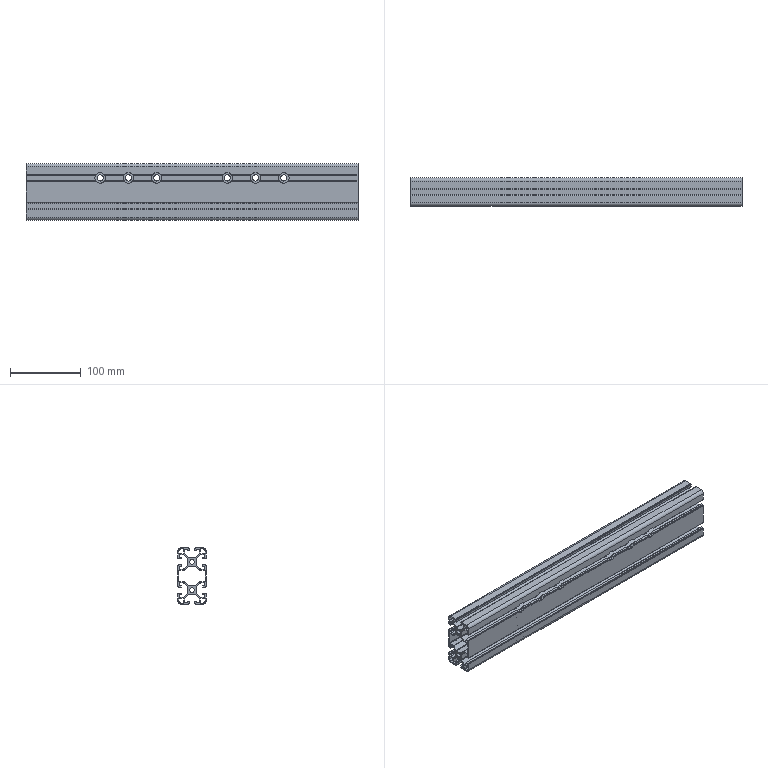Part | STEP file | 1 solid | 556 faces | box 470 x 40 x 80 mm | volume 377061 mm3 | cylinder 324 | plane 232 | commonest cylinder face diameters 0.6 x104 2 x56 4 x40 9 x34 15 x30 0.4 x26